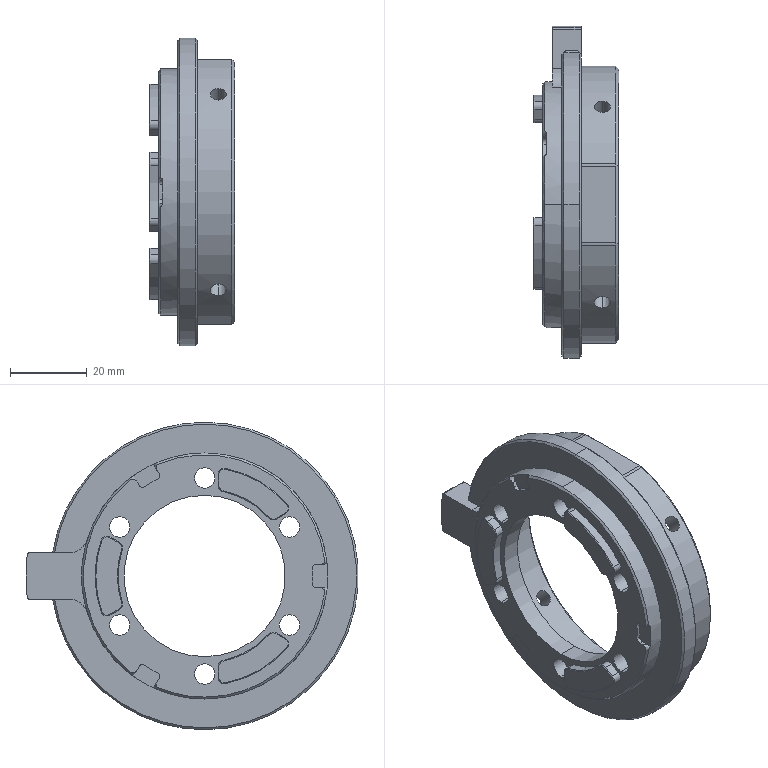CAM job | NX | 3-axis milling, drilling | part box 22.3 x 86.5 x 80 mm | stock box 28.3 x 98.5 x 98.5 mm
Tools:
number,name,description,diameter,corner_radius,flute_length,length,flutes
19,D80,Milling Tool-5 Parameters,80.0,0.0,50.0,75.0,2
15,D10,Milling Tool-5 Parameters,10.0,0.0,50.0,75.0,2
14,D10JING,Milling Tool-5 Parameters,10.0,0.0,50.0,75.0,2
1,D6A45,Milling Tool-5 Parameters,6.0,0.0,50.0,75.0,2
16,5.3ZT,Drilling Tool,5.3,0.0,35.0,50.0,2
17,D4R0.5,Milling Tool-5 Parameters,4.0,0.5,50.0,75.0,2
18,D2,Milling Tool-5 Parameters,2.0,0.0,50.0,75.0,2
Operations:
program,operation,operation_type,tool,method,geometry_group,spindle_rpm,surface_speed,feed_per_tooth,feed_cut,feed_plunge,cut_length_mm,path_length_mm,cut_time_min,machine_time_min
1,FLOOR_WALL,VolumeBased25DMillingOperation,D80,METHOD,A,6500.0,1633.0,0.1154,1500.0,100.0,581.875,635.875,0.3879,0.3933
1,ADAPTIVE_MILLING,CavityMilling,D10,METHOD,A,9500.0,298.0,0.1579,3000.0,1000.0,19681.717,20783.633,7.766,7.876
1,ZLEVEL_PROFILE,ZLevelMilling,D10,METHOD,A,9500.0,298.0,0.1579,3000.0,1000.0,2498.361,2568.041,0.8367,0.8437
1,ZLEVEL_PROFILE_COPY_1_COPY_COPY_1,ZLevelMilling,D10JING,METHOD,A,9500.0,298.0,0.0632,1200.0,1000.0,408.396,715.477,0.3416,0.3723
1,ZLEVEL_PROFILE_COPY_1_COPY_COPY_1_COPY,ZLevelMilling,D10JING,METHOD,A,9500.0,298.0,0.0632,1200.0,1000.0,171.072,254.472,0.1432,0.1515
1,FLOOR_WALL_1,VolumeBased25DMillingOperation,D10JING,METHOD,A,9500.0,298.0,0.0658,1250.0,100.0,449.791,533.391,0.3598,0.3682
1,FLOOR_WALL_1_COPY,VolumeBased25DMillingOperation,D10JING,METHOD,A,9500.0,298.0,0.0658,1250.0,100.0,610.32,683.92,0.4883,0.4956
1,ZLEVEL_PROFILE_1,ZLevelMilling,D4R0.5,METHOD,A,9500.0,119.0,0.1316,2500.0,100.0,4509.554,4594.204,1.804,1.812
1,ZLEVEL_PROFILE_COPY,ZLevelMilling,D2,METHOD,A,9500.0,59.0,0.0526,1000.0,1000.0,481.091,980.509,0.4811,0.531
1,DRILLING,Operation,D6A45,METHOD,A,5000.0,94.0,0.035,350.0,0.0,34.5,301.979,0.0986,0.1253
1,PLANAR_MILL_COPY_COPY_COPY_COPY_COPY_COPY_1,PlanarMilling,D6A45,METHOD,A,9500.0,179.0,0.0658,1250.0,100.0,430.575,556.475,0.3445,0.357
1,PLANAR_MILL_COPY_COPY_COPY_COPY_COPY_COPY_1_COPY,PlanarMilling,D6A45,METHOD,A,9500.0,179.0,0.0658,1250.0,100.0,275.633,355.233,0.2205,0.2285
1,PLANAR_MILL_COPY_COPY_COPY_COPY_COPY_COPY_1_COPY_COPY,PlanarMilling,D6A45,METHOD,A,9500.0,179.0,0.0658,1250.0,100.0,128.245,217.845,0.1026,0.1116
1,DRILLING_COPY,Operation,5.3ZT,METHOD,A,2000.0,33.0,0.05,200.0,0.0,66.554,366.087,0.3328,0.3627
1,TOOLCOMP14,VolumeBased25DMillingOperation,D10JING,METHOD,A,9500.0,298.0,0.0658,1250.0,100.0,262.687,340.287,0.2101,0.2179
2,FLOOR_WALL_COPY,VolumeBased25DMillingOperation,D80,METHOD,B,6500.0,1633.0,0.1154,1500.0,100.0,952.5,1940.501,0.635,0.7338
2,FLOOR_WALL_2,VolumeBased25DMillingOperation,D10,METHOD,B,9500.0,298.0,0.1316,2500.0,1000.0,3661.28,3783.18,1.504,1.516
2,FLOOR_WALL_2_COPY,VolumeBased25DMillingOperation,D10,METHOD,B,9500.0,298.0,0.1316,2500.0,1000.0,566.928,654.572,0.2346,0.2434
2,FLOOR_WALL_2_COPY_COPY,VolumeBased25DMillingOperation,D10,METHOD,B,9500.0,298.0,0.1316,2500.0,1000.0,2642.607,2725.214,1.062,1.07
2,FLOOR_WALL_1_COPY_1,VolumeBased25DMillingOperation,D10JING,METHOD,B,9500.0,298.0,0.0658,1250.0,100.0,903.012,1379.546,0.7224,0.7701
2,FLOOR_WALL_1_COPY_COPY,VolumeBased25DMillingOperation,D10JING,METHOD,B,9500.0,298.0,0.0658,1250.0,100.0,948.934,1276.104,0.7591,0.7919
2,FLOOR_WALL_2_COPY_COPY_COPY,VolumeBased25DMillingOperation,D2,METHOD,B,9500.0,59.0,0.0526,1000.0,1000.0,721.309,1048.4,0.7213,0.754
2,ZLEVEL_PROFILE_1_COPY,ZLevelMilling,D2,METHOD,B,9500.0,59.0,0.0789,1500.0,100.0,860.714,1370.908,0.5738,0.6248
2,PLANAR_MILL_COPY_COPY_COPY_COPY_COPY_COPY_1_COPY_1,PlanarMilling,D6A45,METHOD,B,9500.0,179.0,0.0658,1250.0,100.0,185.696,452.34,0.1486,0.1752
2,PLANAR_MILL_COPY_COPY_COPY_COPY_COPY_COPY_1_COPY_1_COPY,PlanarMilling,D6A45,METHOD,B,9500.0,179.0,0.0658,1250.0,100.0,222.223,285.823,0.1778,0.1841
2,PLANAR_MILL_COPY_COPY_COPY_COPY_COPY_COPY_1_COPY_1_COPY_1,PlanarMilling,D6A45,METHOD,B,9500.0,179.0,0.0658,1250.0,100.0,166.648,894.927,0.1333,0.2061
2,DRILLING_COPY_1,Operation,D6A45,METHOD,B,5000.0,94.0,0.035,350.0,0.0,34.5,277.379,0.0986,0.1229
2,PLANAR_MILL_COPY_COPY_COPY_COPY_COPY_COPY_1_COPY_1_COPY_2,PlanarMilling,D6A45,METHOD,B,9500.0,179.0,0.0658,1250.0,100.0,242.001,316.001,0.1936,0.201
2,PLANAR_MILL_COPY_COPY_COPY_COPY_COPY_COPY_1_COPY_1_COPY_1_COPY,PlanarMilling,D6A45,METHOD,B,9500.0,179.0,0.0658,1250.0,100.0,45.565,115.565,0.0365,0.0435
2,TOOLCOMP14_COPY,VolumeBased25DMillingOperation,D10JING,METHOD,B,9500.0,298.0,0.0658,1250.0,100.0,257.153,533.878,0.2057,0.2334